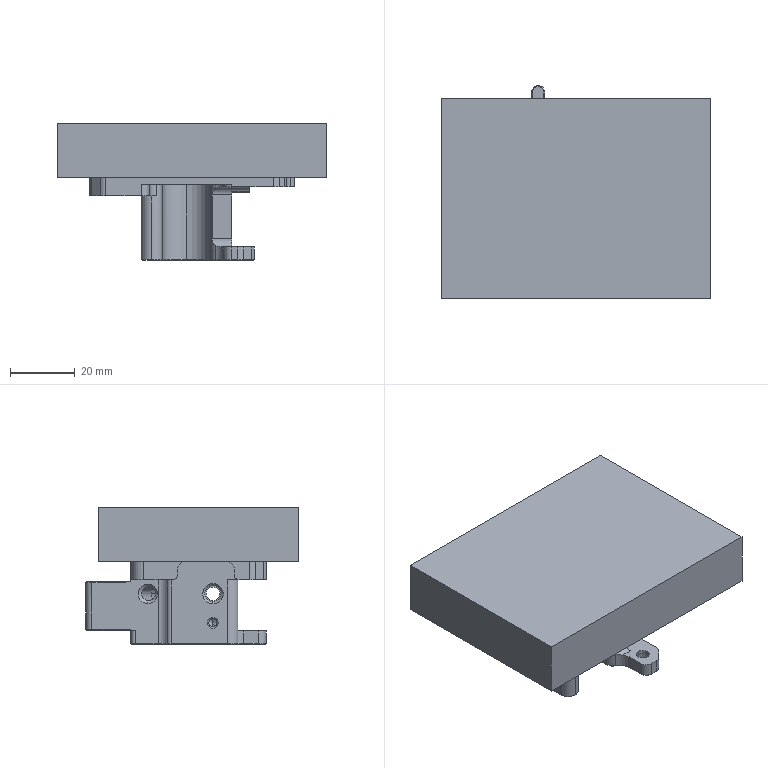NC program | NX | posted with a generic post | part box 83.5 x 66 x 42.45 mm
Whole program:
N10 G17 G21 G94 G90
(ADAPTIVE_MILLING_COPY , TOOL : D10)
N12 T10 M6
N14 G54
N16 G17 G0 G90 X-7.633 Y-11.797 B0. C0. S9500 M3
N18 G43 Z30. H10
N20 Z-19.85
N22 G94 G1 Z-20.85 F1000.
N24 X-5.94 Y-11.706 F3000.
N26 G3 X-4.993 Y-10.829 R1.017
N28 X-4.333 Y-6.187 R16.769
N30 X-4.228 Y3.51 R335.234
N32 G1 X-4.251 Y3.607
N34 X-4.284 Y3.702
N36 X-4.324 Y3.793
N38 X-4.371 Y3.884
N40 X-4.418 Y3.945
N42 X-4.486 Y4.064
N44 X-4.948 Y5.179
N46 X-4.974 Y5.275
N48 G3 X-6.744 Y5.833 R1.102
N50 X-7.136 Y4.797 Z-20.792 R1.208
N52 G1 X-7.132 Y3.95 Z-20.75
N54 X-7.069 Y-9.218
N56 Y-9.799 Z-20.779
N58 X-7.051 Y-10.38 Z-20.808
N60 G3 X-6.632 Y-11.082 Z-20.85 R1.13
N62 X-4.948 Y-10.629 R1.103
N64 X-3.658 Y-5.417 R13.194
N66 X-3.497 Y2.377 R65.836
N68 X-3.689 Y2.995 R2.088
N70 G1 X-4.418 Y3.945
N72 G3 X-5.825 Y4.237 R1.106
N74 X-6.392 Y3.195 Z-20.788 R1.124
N76 G1 X-6.401 Y2.446 Z-20.75
N78 X-6.528 Y-8.058
N80 X-6.529 Y-9.108 Z-20.803
N82 G3 X-6.038 Y-9.886 Z-20.85 R1.117
N84 X-4.486 Y-9.514 R1.104
N86 X-3.183 Y-6.164 R7.051
N88 X-2.791 Y1.51 R34.579
N90 X-3.587 Y2.892 R1.626
N92 G1 X-3.683 Y2.988
N94 X-3.744 Y3.067
N96 G3 X-5.105 Y3.383 R1.106
N98 X-5.72 Y2.355 Z-20.787 R1.123
N100 G1 X-5.753 Y1.621 Z-20.75
N102 X-6.168 Y-7.57
N104 X-6.203 Y-8.599 Z-20.802
N106 G3 X-5.719 Y-9.403 Z-20.85 R1.117
N108 X-4.236 Y-9.157 R1.104
N110 X-2.514 Y-5.381 R7.395
N112 X-2.122 Y0.886 R22.208
N114 X-2.63 Y2.157 R2.042
N116 G1 X-3.264 Y2.644
N118 G3 X-4.502 Y2.713 R1.108
N120 X-5.043 Y1.647 Z-20.787 R1.192
N122 G1 X-5.084 Y0.903 Z-20.75
N124 X-5.511 Y-6.724
N126 X-5.557 Y-7.759 Z-20.802
N128 G3 X-5.087 Y-8.565 Z-20.85 R1.117
N130 X-3.683 Y-8.438 R1.106
N132 X-2.144 Y-5.877 R4.961
N134 X-1.514 Y0.545 R15.572
N136 X-2.116 Y1.884 R2.124
N138 G1 X-2.197 Y1.942
N140 X-2.286 Y1.995
N142 X-2.511 Y2.089
N144 X-2.63 Y2.157
N146 X-2.709 Y2.218
N148 G3 X-3.915 Y2.305 R1.111
N150 X-4.491 Y1.259 Z-20.787 R1.193
N152 G1 X-4.559 Y0.516 Z-20.75
N154 X-5.192 Y-6.428
N156 X-5.276 Y-7.467 Z-20.802
N158 G3 X-4.841 Y-8.285 Z-20.85 R1.117
N160 X-3.508 Y-8.281 R1.108
N162 X-1.571 Y-5.568 R4.957
N164 X-0.975 Y0.436 R11.788
N166 X-1.771 Y1.782 R1.899
N168 G1 X-2.326 Y2.012
N170 G3 X-3.372 Y1.9 R1.115
N172 X-3.861 Y0.924 Z-20.793 R1.217
N174 G1 X-3.955 Y0.064 Z-20.75
N176 X-4.619 Y-5.981
N178 X-4.721 Y-7.021 Z-20.802
N180 G3 X-4.303 Y-7.846 Z-20.85 R1.117
N182 X-2.952 Y-7.854 R1.107
N184 X-0.956 Y-5.176 R5.002
N186 X-0.457 Y0.324 R9.629
N188 X-1.341 Y1.612 R1.726
N190 G1 X-1.397 Y1.627
N192 X-1.858 Y1.818
N194 G3 X-2.954 Y1.671 R1.112
N196 X-3.394 Y0.747 Z-20.797 R1.225
N198 G1 X-3.507 Y-0.188 Z-20.75
N200 X-4.163 Y-5.623
N202 X-4.232 Y-6.163 Z-20.777
N204 X-4.278 Y-6.704 Z-20.804
N206 G3 X-3.885 Y-7.498 Z-20.85 R1.127
N208 X-2.63 Y-7.607 R1.108
N210 X-0.743 Y-5.71 R3.753
N212 X0.048 Y0.209 R8.513
N214 X-0.831 Y1.488 R1.908
N216 G1 X-0.923 Y1.526
N218 X-1.019 Y1.555
N220 X-1.033 Y1.561
N222 X-1.265 Y1.592
N224 X-1.361 Y1.617
N226 G3 X-2.733 Y0.726 R1.103
N228 G1 X-3.834 Y-6.275
N230 G3 X-2.327 Y-7.462 R1.102
N232 X-0.136 Y-5.389 R3.838
N234 X0.494 Y0.234 R7.508
N236 X-0.552 Y1.49 R1.776
N238 G1 X-0.622 Y1.507
N240 X-1.118 Y1.572
N242 G3 X-2.349 Y0.647 R1.104
N244 G1 X-3.373 Y-6.089
N246 G3 X-1.865 Y-7.271 R1.102
N248 X0.473 Y-5.068 R3.97
N250 X0.89 Y0.36 R6.795
N252 X-0.664 Y1.512 R1.595
N254 X-1.897 Y0.57 R1.104
N256 G1 X-2.771 Y-5.866
N258 G3 X-1.397 Y-7.077 R1.102
N260 X0.586 Y-5.61 R3.118
N262 X1.352 Y0.309 R6.494
N264 X0.163 Y1.425 R1.608
N266 G1 X0.034
N268 X-0.034 Y1.429
N270 X-0.232 Y1.456
N272 G3 X-1.462 Y0.542 R1.104
N274 G1 X-2.494 Y-5.773
N276 G3 X-1.265 Y-7.042 R1.103
N278 X0.96 Y-5.68 R2.972
N280 X1.752 Y0.389 R6.179
N282 X0.59 Y1.425 R1.634
N284 G1 X0.09
N286 G3 X-0.994 Y0.517 R1.106
N288 G1 X-2.095 Y-5.707
N290 G3 X-0.868 Y-6.989 R1.103
N292 X1.45 Y-5.598 R3.065
N294 X2.193 Y0.372 R6.012
N296 X1.024 Y1.425 R1.704
N298 G1 X0.524
N300 G3 X-0.56 Y0.508 R1.106
N302 G1 X-1.601 Y-5.65
N304 G3 X-0.372 Y-6.924 R1.103
N306 X1.964 Y-5.486 R3.11
N308 X2.568 Y0.482 R5.809
N310 X0.942 Y1.425 R1.531
N312 X-0.142 Y0.511 R1.106
N314 G1 X-1.19 Y-5.596
N316 G3 X-0.034 Y-6.879 R1.103
N318 X2.175 Y-5.759 R2.764
N320 X2.987 Y0.515 R5.725
N322 X1.354 Y1.425 R1.535
N324 X0.272 Y0.524 R1.106
N326 G1 X-0.848 Y-5.576
N328 G3 X0.234 Y-6.875 R1.103
N330 X2.656 Y-5.708 R2.843
N332 X3.393 Y0.566 R5.65
N334 X1.814 Y1.425 R1.496
N336 X0.734 Y0.534 R1.106
N338 G1 X-0.446 Y-5.566
N340 G3 X0.634 Y-6.875 R1.103
N342 X3.071 Y-5.734 R2.871
N344 X3.852 Y0.532 R5.644
N346 X2.218 Y1.425 R1.527
N348 X1.138 Y0.534 R1.106
N350 G1 X-0.046 Y-5.566
N352 G3 X1.034 Y-6.875 R1.103
N354 X3.552 Y-5.69 R2.935
N356 X4.261 Y0.581 R5.604
N358 X2.681 Y1.425 R1.491
N360 X1.6 Y0.528 R1.106
N362 G1 X0.453 Y-5.572
N364 G3 X1.534 Y-6.875 R1.103
N366 X4.034 Y-5.645 R2.96
N368 X4.674 Y0.631 R5.585
N370 X3.147 Y1.425 R1.463
N372 X2.068 Y0.54 R1.106
N374 G1 X0.855 Y-5.56
N376 G3 X1.934 Y-6.875 R1.103
N378 X4.514 Y-5.604 R2.999
N380 X5.136 Y0.592 R5.596
N382 X3.553 Y1.425 R1.496
N384 X2.475 Y0.541 R1.106
N386 G1 X1.256 Y-5.559
N388 G3 X2.334 Y-6.875 R1.103
N390 X4.93 Y-5.639 R2.977
N392 X5.549 Y0.638 R5.575
N394 X3.957 Y1.425 R1.508
N396 X2.876 Y0.524 R1.106
N398 G1 X1.753 Y-5.576
N400 G3 X2.834 Y-6.875 R1.103
N402 X5.346 Y-5.673 R2.943
N404 X6.015 Y0.601 R5.602
N406 X4.419 Y1.425 R1.498
N408 X3.339 Y0.535 R1.106
N410 G1 X2.155 Y-5.565
N412 G3 X3.234 Y-6.875 R1.103
N414 X5.826 Y-5.629 R2.985
N416 X6.85 Y-3.596 R4.874
N418 X6.793 Y-0.5 R26.04
N420 X5.694 Y1.325 R2.496
N422 X4.909 Y1.425 R2.042
N424 X3.981 Y-0.266 R1.102
N426 G1 X4.822 Y-1.587
N428 G3 X6.85 Y-0.996 R1.101
N430 X6.524 Y0.842 R3.19
N432 X5.228 Y1.425 R1.276
N434 X4.451 Y-0.453 R1.101
N436 G1 X4.772 Y-0.775
N438 X5.104 Y-1.086
N440 G3 X6.85 Y-0.196 R1.101
N442 X6.431 Y1.164 R1.559
N444 X5.612 Y1.425 R1.3
N446 X6.501 Y-0.628 R-1.214
N448 X6.837 Y0.386 R1.243
N450 X6.122 Y1.342 R1.078
N452 G1 X5.147 Y1.12
N454 G3 X4.332 Y0.344 R1.112
N456 G1 X2.707 Y-5.471
N458 G3 X3.027 Y-6.582 R1.112
N460 X4.234 Y-6.872 R1.514
N462 X6.818 Y-4.735 R3.505
N464 X6.85 Y-3.537 R33.415
N466 X4.858 Y-2.893 R1.101
N468 G1 X3.243 Y-5.131
N470 G3 X4.134 Y-6.875 R1.101
N472 X6.782 Y-5.418 R2.78
N474 X6.85 Y-4.522 R3.2
N476 X4.928 Y-3.791 R1.101
N478 G1 X3.813 Y-5.044
N480 G3 X4.634 Y-6.875 R1.101
N482 X6.765 Y-5.853 R2.132
N484 X6.85 Y-5.106 R2.259
N486 X4.999 Y-4.302 R1.101
N488 G1 X4.575 Y-4.694
N490 X4.165 Y-5.101
N492 G3 X5.034 Y-6.875 R1.101
N494 X6.657 Y-6.303 R1.786
N496 X6.85 Y-5.437 R1.428
N498 X4.946 Y-4.686 R1.101
N500 G1 X4.518 Y-5.167
N502 G3 X5.434 Y-6.875 R1.102
N504 X6.84 Y-5.811 R1.191
N506 X6.075 Y-4.697 R1.015
N508 G1 X4.35 Y-4.281
N510 Z-17.85
N512 G0 Z30.
N514 X42.62 Y-2.812
N516 Z-19.85
N518 G1 Z-20.85 F1000.
N520 X40.185 Y-0.632 F3000.
N522 G3 X39.512 Y-0.375 R1.041
N524 X38.91 Y-3.194 R7.946
N526 X38.762 Y-8.987 R44.241
N528 G1 X39.491 Y-10.597
N530 G3 X41.373 Y-10.838 R1.102
N532 X41.574 Y-9.849 Z-20.798 R1.233
N534 G1 X41.465 Y-8.897 Z-20.75
N536 X40.781 Y-2.893
N538 X40.578 Y-1.204 Z-20.835
N540 X40.466 Y-0.928 Z-20.85
N542 G3 X39.512 Y-0.375 R1.112
N544 X38.58 Y-2.336 R4.017
N546 X38.108 Y-8.095 R19.474
N548 G1 X38.13 Y-8.192
N550 X38.161 Y-8.287
N552 X38.2 Y-8.379
N554 X38.246 Y-8.468
N556 X38.278 Y-8.519
N558 X38.896 Y-9.306
N560 G3 X40.86 Y-8.588 R1.101
N562 G1 X40.611 Y-1.437
N564 G3 X39.512 Y-0.375 R1.104
N566 X38.323 Y-1.93 R2.839
N568 X37.518 Y-7.422 R12.095
N570 X38.196 Y-8.415 R1.52
N572 G1 X38.32 Y-8.572
N574 G3 X40.284 Y-7.949 R1.101
N576 G1 X40.61 Y-1.531
N578 G3 X39.512 Y-0.375 R1.104
N580 X38.179 Y-1.509 R2.219
N582 X36.994 Y-6.984 R8.908
N584 X37.391 Y-7.788 R1.417
N586 G1 X37.951 Y-8.209
N588 G3 X39.698 Y-7.496 R1.102
N590 G1 X40.599 Y-1.642
N592 G3 X39.512 Y-0.375 R1.103
N594 X38.012 Y-1.255 R1.989
N596 X36.517 Y-6.7 R7.259
N598 X37.122 Y-7.586 R1.207
N600 G1 X37.442 Y-7.826
N602 G3 X39.172 Y-7.203 R1.102
N604 G1 X40.482 Y-1.731
N606 G3 X39.412 Y-0.375 R1.103
N608 X37.604 Y-1.284 R2.249
N610 X36.054 Y-6.387 R6.419
N612 X37.09 Y-7.568 R1.437
N614 X38.687 Y-6.915 R1.103
N616 G1 X40.169 Y-1.78
N618 G3 X39.112 Y-0.375 R1.103
N620 X37.121 Y-1.358 R2.527
N622 X35.641 Y-6.259 R5.807
N624 X36.777 Y-7.428 R1.47
N626 X38.232 Y-6.752 R1.104
N628 G1 X39.857 Y-1.819
N630 G3 X38.812 Y-0.375 R1.102
N632 X36.633 Y-1.413 R2.73
N634 X35.231 Y-6.123 R5.416
N636 X36.362 Y-7.262 R1.472
N638 X37.805 Y-6.618 R1.104
N640 G1 X39.545 Y-1.852
N642 G3 X38.512 Y-0.375 R1.102
N644 X36.08 Y-1.531 R2.915
N646 X34.855 Y-6.081 R5.051
N648 X35.962 Y-7.101 R1.343
N650 X37.401 Y-6.469 R1.104
N652 G1 X39.141 Y-1.864
N654 G3 X38.112 Y-0.375 R1.102
N656 X35.594 Y-1.569 R2.979
N658 X34.485 Y-6.038 R4.81
N660 X35.721 Y-7.028 R1.3
N662 X36.867 Y-6.359 R1.108
N664 G1 X38.727 Y-1.898
N666 G3 X37.712 Y-0.375 R1.102
N668 X35.111 Y-1.606 R3.015
N670 X34.083 Y-5.902 R4.665
N672 X35.466 Y-6.997 R1.392
N674 X36.631 Y-6.282 R1.106
N676 G1 X38.245 Y-1.852
N678 G3 X37.212 Y-0.375 R1.102
N680 X34.697 Y-1.573 R2.958
N682 X33.788 Y-6.055 R4.474
N684 X35.097 Y-6.953 R1.328
N686 X36.262 Y-6.235 R1.106
N688 G1 X37.846 Y-1.849
N690 G3 X36.812 Y-0.375 R1.102
N692 X34.221 Y-1.618 R2.966
N694 X33.415 Y-6.026 R4.406
N696 X34.776 Y-6.915 R1.379
N698 X35.954 Y-6.161 R1.106
N700 G1 X37.358 Y-1.813
N702 G3 X36.312 Y-0.375 R1.102
N704 X33.811 Y-1.592 R2.908
N706 X33.043 Y-6.002 R4.352
N708 X34.478 Y-6.879 R1.339
N710 X35.592 Y-6.114 R1.107
N712 G1 X36.96 Y-1.808
N714 G3 X35.912 Y-0.375 R1.103
N716 X33.282 Y-1.728 R2.926
N718 X32.766 Y-6.161 R4.226
N720 X34.115 Y-6.875 R1.284
N722 X35.168 Y-6.093 R1.108
N724 G1 X36.465 Y-1.793
N726 G3 X35.412 Y-0.375 R1.103
N728 X32.938 Y-1.633 R2.829
N730 X32.399 Y-6.148 R4.222
N732 X33.748 Y-6.875 R1.29
N734 X34.804 Y-6.085 R1.108
N736 G1 X36.067 Y-1.785
N738 G3 X35.012 Y-0.375 R1.103
N740 X32.537 Y-1.624 R2.8
N742 X32.076 Y-6.225 R4.166
N744 X33.031 Y-6.875 R1.276
N746 X34.064 Y-6.154 R1.108
N748 G1 X35.644 Y-1.855
N750 G3 X34.612 Y-0.375 R1.102
N752 X32.138 Y-1.619 R2.763
N754 X31.706 Y-6.225 R4.175
N756 X32.66 Y-6.875 R1.273
N758 G1 X33.36
N760 G3 X34.444 Y-5.964 R1.106
N762 G1 X35.195 Y-1.664
N764 G3 X34.112 Y-0.375 R1.103
N766 X31.801 Y-1.537 R2.68
N768 X31.335 Y-6.227 R4.202
N770 X32.291 Y-6.875 R1.282
N772 X33.336 Y-6.12 R1.108
N774 G1 X34.756 Y-1.82
N776 G3 X33.712 Y-0.375 R1.102
N778 X31.34 Y-1.615 R2.704
N780 X31.015 Y-6.31 R4.153
N782 X31.916 Y-6.875 R1.238
N784 X32.962 Y-6.115 R1.108
N786 G1 X34.358 Y-1.815
N788 G3 X33.312 Y-0.375 R1.102
N790 X30.941 Y-1.616 R2.695
N792 X30.15 Y-3.468 R4.553
N794 X30.361 Y-5.743 R6.35
N796 X31.475 Y-6.875 R1.607
N798 G1 X32.675
N800 G3 X33.774 Y-5.835 R1.104
N802 G1 X34.01 Y-1.535
N804 G3 X32.912 Y-0.375 R1.104
N806 X30.685 Y-1.44 R2.524
N808 X30.15 Y-2.478 R2.062
N810 G1 Y-3.478
N812 G3 X32.172 Y-4.077 R1.101
N814 G1 X33.484 Y-2.058
N816 G3 X32.633 Y-0.361 R1.102
N818 X30.191 Y-1.722 R2.337
N820 X30.15 Y-2.535 R7.597
N822 X32.097 Y-3.237 R1.101
N824 G1 X32.613 Y-2.623
N826 X33.109 Y-1.993
N828 G3 X32.234 Y-0.335 R1.102
N830 X30.201 Y-1.334 R1.806
N832 X30.15 Y-1.996 R2.134
N834 X32.084 Y-2.713 R1.101
N836 G1 X32.407 Y-2.34
N838 X32.716 Y-1.956
N840 G3 X31.99 Y-0.302 R1.102
N842 X30.159 Y-1.2 R1.423
N844 G1 X30.15 Y-1.315
N846 Y-1.515
N848 G3 X31.695 Y-0.244 R-1.295
N850 X30.155 Y-1.255 R1.153
N852 X32.247 Y-1.34 R-1.047
N854 X30.921 Y-0.241 R1.094
N856 X30.162 Y-1.155 R1.124
N858 G1 X30.15 Y-1.315
N860 Y-4.568
N862 G3 X30.365 Y-6.233 R3.413
N864 X31.488 Y-6.875 R1.101
N866 X32.357 Y-5.101 R1.101
N868 G1 X31.996 Y-4.66
N870 G3 X30.15 Y-5.468 R1.101
N872 X31.115 Y-6.852 R1.188
N874 X32.223 Y-6.109 R1.015
N876 G1 X32.682 Y-4.375
N878 Z-17.85
N880 G0 Z30.
N882 X33.104 Y-2.875
N884 Z-18.35
N886 G1 Z-19.35 F1000.
N888 X31.654 Y-0.499 F3000.
N890 G3 X31.163 Y-0.086 R1.052
N892 X29.911 Y-0.971 R1.106
N894 X29.52 Y-5.518 R10.628
N896 X30.478 Y-6.827 R1.624
N898 G1 X30.575 Y-6.852
N900 X30.673 Y-6.87
N902 X30.693 Y-6.875
N904 X30.893
N906 G3 X31.992 Y-5.743 R1.104
N908 G1 X31.858 Y-1.078
N910 G3 X31.163 Y-0.086 R1.108
N912 X29.892 Y-0.598 R1.041
N914 X29.125 Y-5.603 R6.555
N916 X30.18 Y-6.843 R1.696
N918 G1 X30.278 Y-6.864
N920 X30.314 Y-6.875
N922 X30.714
N924 G3 X31.814 Y-5.764 R1.104
N926 G1 X31.766 Y-1.061
N928 G3 X31.071 Y-0.049 R1.108
N930 X29.743 Y-0.481 R1.168
N932 X28.815 Y-5.841 R5.414
N934 X30.361 Y-6.875 R1.469
N936 X31.46 Y-5.824 R1.104
N938 G1 X31.672 Y-1.085
N940 G3 X30.978 Y-0.013 R1.108
N942 X29.524 Y-0.411 R1.358
N944 X28.519 Y-6.041 R4.94
N946 X29.984 Y-6.875 R1.396
N948 X31.078 Y-5.889 R1.106
N950 G1 X31.574 Y-1.112
N952 G3 X30.885 Y0.024 R1.108
N954 X29.309 Y-0.301 R1.492
N956 X28.164 Y-6.116 R4.763
N958 X29.6 Y-6.875 R1.368
N960 X30.689 Y-5.931 R1.106
N962 G1 X31.383 Y-1.081
N964 G3 X30.699 Y0.098 R1.106
N966 X29.016 Y-0.225 R1.662
N968 X27.795 Y-6.171 R4.709
N970 X29.208 Y-6.875 R1.357
N972 X30.29 Y-5.973 R1.106
N974 G1 X31.19 Y-1.049
N976 G3 X30.513 Y0.171 R1.106
N978 X28.724 Y-0.13 R1.813
N980 X27.42 Y-6.21 R4.682
N982 X28.899 Y-6.875 R1.443
N984 X29.977 Y-5.996 R1.106
N986 G1 X31. Y-0.998
N988 G3 X30.327 Y0.245 R1.106
N990 X28.392 Y-0.042 R1.938
N992 X26.95 Y-6.104 R4.744
N994 X28.4 Y-6.875 R1.384
N996 X29.468 Y-6.039 R1.107
N998 G1 X30.732 Y-0.932
N1000 G3 X30.187 Y0.3 R1.107
N1002 X28.353 Y0.234 R1.818
N1004 X26.554 Y-6.12 R4.77
N1006 X28.094 Y-6.875 R1.458
N1008 X29.159 Y-6.05 R1.107
N1010 G1 X30.509 Y-0.814
N1012 G3 X30.078 Y0.359 R1.108
N1014 X28.272 Y0.469 R1.761
N1016 X25.602 Y-3.585 R4.701
N1018 X26.497 Y-6.561 R3.849
N1020 X27.595 Y-6.875 R1.385
N1022 X28.645 Y-6.105 R1.108
N1024 G1 X30.329 Y-0.754
N1026 G3 X29.915 Y0.475 R1.108
N1028 X27.921 Y0.602 R1.932
N1030 X25.17 Y-3.93 R4.894
N1032 X26.198 Y-6.655 R3.571
N1034 X27.277 Y-6.875 R1.642
N1036 X28.319 Y-6.126 R1.108
N1038 G1 X30.159 Y-0.66
N1040 G3 X29.751 Y0.59 R1.108
N1042 X27.668 Y0.786 R2.019
N1044 X24.751 Y-3.756 R5.003
N1046 X25.728 Y-6.607 R3.797
N1048 X26.865 Y-6.875 R1.56
N1050 X27.901 Y-6.144 R1.108
N1052 G1 X29.908 Y-0.504
N1054 G3 X29.506 Y0.763 R1.108
N1056 X27.42 Y0.978 R2.06
N1058 X24.358 Y-3.266 R5.054
N1060 X25.248 Y-6.542 R4.104
N1062 X26.457 Y-6.875 R1.491
N1064 X27.488 Y-6.16 R1.108
N1066 G1 X29.657 Y-0.347
N1068 G3 X29.261 Y0.936 R1.107
N1070 X27.078 Y1.147 R2.161
N1072 X23.903 Y-3.562 R5.236
N1074 X24.9 Y-6.607 R3.925
N1076 X26.037 Y-6.875 R1.56
N1078 X27.061 Y-6.176 R1.108
N1080 G1 X29.406 Y-0.191
N1082 G3 X29.016 Y1.109 R1.107
N1084 X28.201 Y1.425 R1.402
N1086 X24.604 Y-0.338 R3.962
N1088 X24.004 Y-6.003 R5.379
N1090 X25.634 Y-6.875 R1.506
N1092 X26.686 Y-6.097 R1.108
N1094 G1 X28.553 Y0.003
N1096 G3 X27.501 Y1.425 R1.103
N1098 X24.366 Y-0.02 R3.589
N1100 X23.539 Y-5.925 R5.498
N1102 X25.205 Y-6.875 R1.528
N1104 X26.264 Y-6.07 R1.108
N1106 G1 X27.961 Y0.03
N1108 G3 X26.901 Y1.425 R1.103
N1110 X23.945 Y0.051 R3.398
N1112 X23.122 Y-5.945 R5.532
N1114 X24.777 Y-6.875 R1.529
N1116 X25.844 Y-6.042 R1.107
N1118 G1 X27.368 Y0.058
N1120 G3 X26.301 Y1.425 R1.103
N1122 X23.523 Y0.111 R3.261
N1124 X22.659 Y-5.886 R5.604
N1126 X24.343 Y-6.875 R1.563
N1128 X25.413 Y-6.031 R1.106
N1130 G1 X26.871 Y0.069
N1132 G3 X25.801 Y1.425 R1.103
N1134 X23.103 Y0.164 R3.171
N1136 X22.245 Y-5.919 R5.603
N1138 X23.924 Y-6.875 R1.549
N1140 X24.998 Y-6.017 R1.106
N1142 G1 X26.374 Y0.083
N1144 G3 X25.301 Y1.425 R1.103
N1146 X22.684 Y0.213 R3.093
N1148 X21.831 Y-5.954 R5.594
N1150 X23.482 Y-6.875 R1.532
N1152 X24.557 Y-6.007 R1.106
N1154 G1 X25.876 Y0.093
N1156 G3 X24.801 Y1.425 R1.103
N1158 X22.2 Y0.184 R3.074
N1160 X21.419 Y-5.99 R5.576
N1162 X23.053 Y-6.875 R1.516
N1164 X24.131 Y-5.995 R1.106
N1166 G1 X25.379 Y0.105
N1168 G3 X24.301 Y1.425 R1.103
N1170 X21.78 Y0.227 R3.03
N1172 X21.006 Y-6.032 R5.578
N1174 X22.614 Y-6.875 R1.5
N1176 X23.69 Y-6.002 R1.106
N1178 G1 X24.977 Y0.098
N1180 G3 X23.901 Y1.425 R1.103
N1182 X21.297 Y0.194 R3.043
N1184 X20.542 Y-5.987 R5.605
N1186 X22.176 Y-6.875 R1.521
N1188 X23.255 Y-5.992 R1.106
N1190 G1 X24.48 Y0.108
N1192 G3 X23.401 Y1.425 R1.103
N1194 X20.88 Y0.233 R3.004
N1196 X20.13 Y-6.031 R5.59
N1198 X21.742 Y-6.875 R1.506
N1200 X22.819 Y-5.997 R1.106
N1202 G1 X24.078 Y0.103
N1204 G3 X23.001 Y1.425 R1.103
N1206 X20.398 Y0.196 R3.025
N1208 X19.667 Y-5.989 R5.617
N1210 X21.302 Y-6.875 R1.525
N1212 X22.382 Y-5.987 R1.106
N1214 G1 X23.58 Y0.113
N1216 G3 X22.501 Y1.425 R1.103
N1218 X19.916 Y0.157 R3.031
N1220 X19.255 Y-6.034 R5.588
N1222 X20.866 Y-6.875 R1.508
N1224 X21.944 Y-5.993 R1.106
N1226 G1 X23.179 Y0.107
N1228 G3 X22.101 Y1.425 R1.103
N1230 X19.5 Y0.192 R3.018
N1232 X18.845 Y-6.08 R5.573
N1234 X20.432 Y-6.875 R1.502
N1236 X21.512 Y-5.982 R1.106
N1238 G1 X22.681 Y0.118
N1240 G3 X21.601 Y1.425 R1.103
N1242 X19.084 Y0.227 R2.983
N1244 X18.381 Y-6.042 R5.591
N1246 X19.987 Y-6.875 R1.508
N1248 X21.066 Y-5.99 R1.106
N1250 G1 X22.28 Y0.11
N1252 G3 X21.201 Y1.425 R1.103
N1254 X18.603 Y0.189 R3.011
N1256 X17.917 Y-6.001 R5.618
N1258 X19.559 Y-6.875 R1.524
N1260 X20.64 Y-5.977 R1.106
N1262 G1 X21.782 Y0.123
N1264 G3 X20.701 Y1.425 R1.103
N1266 X18.187 Y0.224 R2.972
N1268 X17.505 Y-6.049 R5.598
N1270 X19.106 Y-6.875 R1.505
N1272 X20.185 Y-5.986 R1.106
N1274 G1 X21.381 Y0.114
N1276 G3 X20.301 Y1.425 R1.103
N1278 X17.707 Y0.183 R3.001
N1280 X17.041 Y-6.009 R5.603
N1282 X18.677 Y-6.875 R1.521
N1284 X19.759 Y-5.974 R1.106
N1286 G1 X20.883 Y0.126
N1288 G3 X19.801 Y1.425 R1.103
N1290 X17.292 Y0.216 R2.959
N1292 X16.028 Y-2.678 R5.781
N1294 X18.007 Y-3.488 R1.101
N1296 G1 X20.293 Y-0.318
N1298 G3 X19.401 Y1.425 R1.101
N1300 X16.812 Y0.175 R2.981
N1302 X16.031 Y-1.1 R6.798
N1304 X17.815 Y-2.324 R1.1
N1306 G1 X19.68 Y-0.451
N1308 G3 X18.901 Y1.425 R1.101
N1310 X16.396 Y0.208 R2.953
N1312 G1 X16.332 Y0.131
N1314 X16.271 Y0.052
N1316 X16.212 Y-0.028
N1318 X16.155 Y-0.111
N1320 X16.101 Y-0.195
N1322 X16.05 Y-0.281
N1324 X16.005 Y-0.371
N1326 X15.951 Y-0.454
N1328 X15.887 Y-0.531
N1330 X15.815 Y-0.601
N1332 G2 X13.693 Y-1.037 R3.605
N1334 X9.481 Y0.413 R9.233
N1336 G3 X7.632 Y1.399 R13.696
N1338 G1 X7.534 Y1.418
N1340 X7.47 Y1.425
N1342 X6.07
N1344 G3 X5.314 Y-0.255 R1.011
N1346 G1 X5.584 Y-0.561
N1348 X5.866 Y-0.857
N1350 G3 X6.498 Y-1.079 R1.05
N1352 G1 Z-16.35
N1354 G0 Z30.
N1356 X18.779 Y-1.087
N1358 Z-18.35
N1360 G1 Z-19.35 F1000.
N1362 G3 X19.659 Y0.42 R1.012 F3000.
N1364 G1 X19.296 Y1.039
N1366 G3 X18.501 Y1.425 R1.026
N1368 X16.855 Y1.087 R3.428
N1370 G2 X11.338 Y1.163 R9.468
N1372 G1 X11.049 Y1.243
N1374 X10.568 Y1.381
N1376 X10.471 Y1.405
N1378 X10.373 Y1.422
N1380 X10.342 Y1.425
N1382 X7.442
N1384 G3 X6.344 Y0.323 R1.1
N1386 X7.442 Y-0.775 R1.1
N1388 G1 X18.001
N1390 G3 X19.099 Y0.327 R1.1
N1392 X18.001 Y1.425 R1.1
N1394 G1 X10.301
N1396 G3 X9.393 Y0.946 R1.116
N1398 G1 X5.223 Y-5.154
N1400 G3 X6.131 Y-6.875 R1.101
N1402 X6.991 Y-6.128 R1.118
N1404 G2 X8.68 Y-4.837 R2.414
N1406 X13.443 Y-5.402 R6.92
N1408 G1 X13.534 Y-5.443
N1410 X13.715 Y-5.527
N1412 X13.985 Y-5.658
N1414 X14.253 Y-5.793
N1416 X14.519 Y-5.932
N1418 X14.872 Y-6.12
N1420 X15.136 Y-6.262
N1422 X15.401 Y-6.403
N1424 X15.579 Y-6.495
N1426 X15.757 Y-6.586
N1428 X15.846 Y-6.631
N1430 X16.027 Y-6.718
N1432 X16.117 Y-6.759
N1434 X16.209 Y-6.8
N1436 X16.304 Y-6.832
N1438 G3 X18.227 Y-6.875 R12.574
N1440 X19.325 Y-5.773 R1.1
N1442 X18.227 Y-4.675 R1.1
N1444 G1 X6.131
N1446 G3 X5.033 Y-5.777 R1.1
N1448 X6.131 Y-6.875 R1.1
N1450 X7.182 Y-6.581 R3.325
N1452 G2 X12.804 Y-6.695 R10.069
N1454 G1 X13.094 Y-6.772
N1456 X13.383 Y-6.851
N1458 X13.481 Y-6.869
N1460 X13.538 Y-6.875
N1462 X16.538
N1464 G3 X17.636 Y-5.773 R1.1
N1466 X16.538 Y-4.675 R1.1
N1468 G1 X6.231
N1470 G3 X5.133 Y-5.777 R1.1
N1472 X6.231 Y-6.875 R1.1
N1474 G1 X13.631
N1476 G3 X14.63 Y-5.716 R1.014
N1478 G1 X14.447 Y-4.485
N1480 Z-16.35
N1482 G0 Z30.
N1484 X39.329 Y-1.071
N1486 Z-12.482
N1488 G1 Z-13.482 F1000.
N1490 X39.004 Y0.607 F3000.
N1492 G3 X38.012 Y1.425 R1.017
N1494 G2 X31.62 Y1.402 R10.217
N1496 G1 X31.521 Y1.42
N1498 X31.473 Y1.425
N1500 X28.473
N1502 G3 X27.375 Y0.323 R1.1
N1504 X28.473 Y-0.775 R1.1
N1506 G1 X38.012
N1508 G3 X39.11 Y0.327 R1.1
N1510 X38.012 Y1.425 R1.1
N1512 G1 X31.412
N1514 G3 X30.408 Y0.521 R1.015
N1516 G1 X30.24 Y-1.072
N1518 Z-10.482
N1520 G0 Z30.
N1522 M5
(DRILLING_COPY_1_COPY_COPY , TOOL : D4A45)
N1524 T07 M6
N1526 G54
N1528 G17 G0 G90 X16.52 Y-0.525 B0. C0. S5000 M3
N1530 G43 Z30. H7
N1532 G94 G81 G98 Z-21.15 F250. R-16.5
N1534 G80
N1536 G0 X16.52 Y-0.525 Z30.
N1538 M5
(DRILLING_COPY_COPY_1_1_COPY_COPY , TOOL : 4.2ZT)
N1540 T14 M6
N1542 G54
N1544 G17 G0 G90 X16.52 Y-0.525 B0. C0. S2000 M3
N1546 G43 Z30. H14
N1548 G94 G83 G98 Z-28.762 F120. Q2. R-16.5
N1550 G80
N1552 G0 X16.52 Y-0.525 Z30.
N1554 M5
(ZLEVEL_PROFILE_COPY_1_COPY_1_COPY_1_1_COPY_COPY_COPY_1_COPY_1 , TOOL : D4)
N1556 T04 M6
N1558 G54
N1560 G17 G0 G90 X31.192 Y2.422 B0. C0. S9500 M3
N1562 G43 Z30. H4
N1564 Z-14.4
N1566 G94 G1 X31.316 Y3.026 F800.
N1568 G3 X31.189 Y3.406 R0.4
N1570 G2 X30.558 Y4.275 R2.5 F1400.
N1572 G3 X30.1 Y4.575 R0.5
N1574 G1 X28.627
N1576 G3 X28.281 Y4.375 R0.4
N1578 G1 X27.934 Y3.775
N1580 G0 X31.192 Y2.422 Z-14.8
N1582 G1 X31.316 Y3.026 F800.
N1584 G3 X31.189 Y3.406 R0.4
N1586 G2 X30.558 Y4.275 R2.5 F1400.
N1588 G3 X30.1 Y4.575 R0.5
N1590 G1 X28.627
N1592 G3 X28.281 Y4.375 R0.4
N1594 G1 X27.934 Y3.775
N1596 G0 X31.192 Y2.422 Z-15.2
N1598 G1 X31.316 Y3.026 F800.
N1600 G3 X31.189 Y3.406 R0.4
N1602 G2 X30.558 Y4.275 R2.5 F1400.
N1604 G3 X30.1 Y4.575 R0.5
N1606 G1 X28.627
N1608 G3 X28.281 Y4.375 R0.4
N1610 G1 X27.934 Y3.775
N1612 G0 X31.192 Y2.422 Z-15.6
N1614 G1 X31.316 Y3.026 F800.
N1616 G3 X31.189 Y3.406 R0.4
N1618 G2 X30.558 Y4.275 R2.5 F1400.
N1620 G3 X30.1 Y4.575 R0.5
N1622 G1 X28.627
N1624 G3 X28.281 Y4.375 R0.4
N1626 G1 X27.934 Y3.775
N1628 G0 X31.192 Y2.422 Z-16.
N1630 G1 X31.316 Y3.026 F800.
N1632 G3 X31.189 Y3.406 R0.4
N1634 G2 X30.558 Y4.275 R2.5 F1400.
N1636 G3 X30.1 Y4.575 R0.5
N1638 G1 X28.627
N1640 G3 X28.281 Y4.375 R0.4
N1642 G1 X27.934 Y3.775
N1644 G0 X31.192 Y2.422 Z-16.4
N1646 G1 X31.316 Y3.026 F800.
N1648 G3 X31.189 Y3.406 R0.4
N1650 G2 X30.558 Y4.275 R2.5 F1400.
N1652 G3 X30.1 Y4.575 R0.5
N1654 G1 X28.627
N1656 G3 X28.281 Y4.375 R0.4
N1658 G1 X27.934 Y3.775
N1660 G0 X31.192 Y2.422 Z-16.8
N1662 G1 X31.316 Y3.026 F800.
N1664 G3 X31.189 Y3.406 R0.4
N1666 G2 X30.558 Y4.275 R2.5 F1400.
N1668 G3 X30.1 Y4.575 R0.5
N1670 G1 X28.627
N1672 G3 X28.281 Y4.375 R0.4
N1674 G1 X27.934 Y3.775
N1676 G0 X31.192 Y2.422 Z-17.199
N1678 G1 X31.316 Y3.026 F800.
N1680 G3 X31.189 Y3.406 R0.4
N1682 G2 X30.558 Y4.275 R2.5 F1400.
N1684 G3 X30.1 Y4.575 R0.5
N1686 G1 X28.627
N1688 G3 X28.281 Y4.375 R0.4
N1690 G1 X27.934 Y3.775
N1692 G0 X31.192 Y2.422 Z-17.599
N1694 G1 X31.316 Y3.026 F800.
N1696 G3 X31.189 Y3.406 R0.4
N1698 G2 X30.558 Y4.275 R2.5 F1400.
N1700 G3 X30.1 Y4.575 R0.5
N1702 G1 X28.627
N1704 G3 X28.281 Y4.375 R0.4
N1706 G1 X27.934 Y3.775
N1708 G0 X31.192 Y2.422 Z-17.999
N1710 G1 X31.316 Y3.026 F800.
N1712 G3 X31.189 Y3.406 R0.4
N1714 G2 X30.558 Y4.275 R2.5 F1400.
N1716 G3 X30.1 Y4.575 R0.5
N1718 G1 X28.627
N1720 G3 X28.281 Y4.375 R0.4
N1722 G1 X27.934 Y3.775
N1724 G0 X31.192 Y2.422 Z-18.375
N1726 G1 X31.316 Y3.026 F800.
N1728 G3 X31.189 Y3.406 R0.4
N1730 G2 X30.558 Y4.275 R2.5 F1400.
N1732 G3 X30.1 Y4.575 R0.5
N1734 G1 X28.627
N1736 G3 X28.281 Y4.375 R0.4
N1738 G1 X27.934 Y3.775
N1740 G0 X31.192 Y2.422 Z-18.75
N1742 G1 X31.316 Y3.026 F800.
N1744 G3 X31.189 Y3.406 R0.4
N1746 G2 X30.558 Y4.275 R2.5 F1400.
N1748 G3 X30.1 Y4.575 R0.5
N1750 G1 X28.627
N1752 G3 X28.281 Y4.375 R0.4
N1754 G1 X27.934 Y3.775
N1756 G0 X31.192 Y2.422 Z-19.125
N1758 G1 X31.316 Y3.026 F800.
N1760 G3 X31.189 Y3.406 R0.4
N1762 G2 X30.558 Y4.275 R2.5 F1400.
N1764 G3 X30.1 Y4.575 R0.5
N1766 G1 X28.627
N1768 G3 X28.281 Y4.375 R0.4
N1770 G1 X27.934 Y3.775
N1772 G0 X31.192 Y2.422 Z-19.5
N1774 G1 X31.316 Y3.026 F800.
N1776 G3 X31.189 Y3.406 R0.4
N1778 G2 X30.558 Y4.275 R2.5 F1400.
N1780 G3 X30.1 Y4.575 R0.5
N1782 G1 X28.627
N1784 G3 X28.281 Y4.375 R0.4
N1786 G1 X27.934 Y3.775
N1788 G0 X32.071 Y2.068 Z-19.85
N1790 G1 X32.018 Y2.683 F800.
N1792 G3 X31.789 Y3.011 R0.4
N1794 G2 X30.558 Y4.275 R2.5 F1400.
N1796 G3 X30.1 Y4.575 R0.5
N1798 G1 X27.5
N1800 G3 X27. Y4.075 R0.5
N1802 G1 Y0.418
N1804 G3 X27.2 Y0.071 R0.4
N1806 G1 X27.8 Y-0.275
N1808 G0 X32.071 Y2.068 Z-20.177
N1810 G1 X32.018 Y2.683 F800.
N1812 G3 X31.789 Y3.011 R0.4
N1814 G2 X30.558 Y4.275 R2.5 F1400.
N1816 G3 X30.1 Y4.575 R0.5
N1818 G1 X27.5
N1820 G3 X27. Y4.075 R0.5
N1822 G1 Y0.418
N1824 G3 X27.2 Y0.071 R0.4
N1826 G1 X27.8 Y-0.275
N1828 G0 X32.071 Y2.068 Z-20.474
N1830 G1 X32.018 Y2.683 F800.
N1832 G3 X31.789 Y3.011 R0.4
N1834 G2 X30.558 Y4.275 R2.5 F1400.
N1836 G3 X30.1 Y4.575 R0.5
N1838 G1 X27.5
N1840 G3 X27. Y4.075 R0.5
N1842 G1 Y0.418
N1844 G3 X27.2 Y0.071 R0.4
N1846 G1 X27.8 Y-0.275
N1848 G0 X32.071 Y2.068 Z-20.74
N1850 G1 X32.018 Y2.683 F800.
N1852 G3 X31.789 Y3.011 R0.4
N1854 G2 X30.558 Y4.275 R2.5 F1400.
N1856 G3 X30.1 Y4.575 R0.5
N1858 G1 X27.5
N1860 G3 X27. Y4.075 R0.5
N1862 G1 Y0.418
N1864 G3 X27.2 Y0.071 R0.4
N1866 G1 X27.8 Y-0.275
N1868 G0 X32.071 Y2.068 Z-20.879
N1870 G1 X32.018 Y2.683 F800.
N1872 G3 X31.789 Y3.011 R0.4
N1874 G2 X30.558 Y4.275 R2.5 F1400.
N1876 G3 X30.1 Y4.575 R0.5
N1878 G1 X27.5
N1880 G3 X27. Y4.075 R0.5
N1882 G1 Y0.418
N1884 G3 X27.2 Y0.071 R0.4
N1886 G1 X27.8 Y-0.275
N1888 G0 X32.071 Y2.068 Z-21.
N1890 G1 X32.018 Y2.683 F800.
N1892 G3 X31.789 Y3.011 R0.4
N1894 G2 X30.558 Y4.275 R2.5 F1400.
N1896 G3 X30.1 Y4.575 R0.5
N1898 G1 X27.5
N1900 G3 X27. Y4.075 R0.5
N1902 G1 Y0.418
N1904 G3 X27.2 Y0.071 R0.4
N1906 G1 X27.8 Y-0.275
N1908 G0 Z30.
N1910 Y-6.179
N1912 Z-19.85
N1914 G1 X27.2 Y-6.526 F800.
N1916 G3 X27. Y-6.872 R0.4
N1918 G1 Y-9.525 F1400.
N1920 G3 X27.5 Y-10.025 R0.5
N1922 G1 X30.153
N1924 G3 X30.499 Y-9.825 R0.4
N1926 G1 X30.846 Y-9.225
N1928 G0 X27.8 Y-6.179 Z-20.177
N1930 G1 X27.2 Y-6.526 F800.
N1932 G3 X27. Y-6.872 R0.4
N1934 G1 Y-9.525 F1400.
N1936 G3 X27.5 Y-10.025 R0.5
N1938 G1 X30.153
N1940 G3 X30.499 Y-9.825 R0.4
N1942 G1 X30.846 Y-9.225
N1944 G0 X27.8 Y-6.179 Z-20.474
N1946 G1 X27.2 Y-6.526 F800.
N1948 G3 X27. Y-6.872 R0.4
N1950 G1 Y-9.525 F1400.
N1952 G3 X27.5 Y-10.025 R0.5
N1954 G1 X30.153
N1956 G3 X30.499 Y-9.825 R0.4
N1958 G1 X30.846 Y-9.225
N1960 G0 X27.8 Y-6.179 Z-20.74
N1962 G1 X27.2 Y-6.526 F800.
N1964 G3 X27. Y-6.872 R0.4
N1966 G1 Y-9.525 F1400.
N1968 G3 X27.5 Y-10.025 R0.5
N1970 G1 X30.153
N1972 G3 X30.499 Y-9.825 R0.4
N1974 G1 X30.846 Y-9.225
N1976 G0 X27.8 Y-6.179 Z-20.879
N1978 G1 X27.2 Y-6.526 F800.
N1980 G3 X27. Y-6.872 R0.4
N1982 G1 Y-9.525 F1400.
N1984 G3 X27.5 Y-10.025 R0.5
N1986 G1 X30.153
N1988 G3 X30.499 Y-9.825 R0.4
N1990 G1 X30.846 Y-9.225
N1992 G0 X27.8 Y-6.179 Z-21.
N1994 G1 X27.2 Y-6.526 F800.
N1996 G3 X27. Y-6.872 R0.4
N1998 G1 Y-9.525 F1400.
N2000 G3 X27.5 Y-10.025 R0.5
N2002 G1 X30.153
N2004 G3 X30.499 Y-9.825 R0.4
N2006 G1 X30.846 Y-9.225
N2008 G0 Z30.
(FLOOR_WALL_1_1_COPY_1_COPY , TOOL : D4)
N2010 X43.418 Y1.588
N2012 Z-12.5
N2014 G1 Z-14. F1000.
N2016 X42.846 Y2.578
N2018 G3 X42.5 Y2.778 R0.4
N2020 G1 X32.727
N2022 G2 X30.5 Y4.375 R2.548
N2024 G1 X42.5
N2026 G2 X42.846 Y4.175 R0.4
N2028 G1 X43.925 Y2.307
N2030 Z-12.5
N2032 G0 Z30.
N2034 X43.963 Y2.442
N2036 Z-12.5
N2038 G1 Z-14.
N2040 X42.846 Y4.375
N2042 G3 X42.5 Y4.575 R0.4
N2044 G1 X30.276
N2046 G3 X29.929 Y4.375 R0.4
N2048 G1 X29.179 Y3.075
N2050 Z-12.5
N2052 G0 Z30.
N2054 X38.197 Y1.275
N2056 Z-19.5
N2058 G1 Z-21.
N2060 X36.497 Y2.229
N2062 G3 X36.697 Y2.575 R0.4
N2064 G1 Y-9.825
N2066 X34.798
N2068 Y2.575
N2070 X32.898
N2072 Y-9.825
N2074 X30.999
N2076 Y3.309
N2078 G2 X30.375 Y4.195 R2.7
N2080 G3 X30.1 Y4.375 R0.3
N2082 G1 X29.099
N2084 Y-9.825
N2086 X27.5
N2088 G2 X27.2 Y-9.528 R0.3
N2090 G1 Y4.078
N2092 G2 X27.3 Y4.251 R0.2
N2094 G1 Z-19.5
N2096 G0 Z30.
N2098 X38.197 Y0.577
N2100 Z-19.5
N2102 G1 Z-21.
N2104 X37.044 Y2.575
N2106 G3 X36.697 Y2.775 R0.4
N2108 G1 X32.85
N2110 G2 X30.558 Y4.275 R2.5
N2112 G3 X30.1 Y4.575 R0.5
N2114 G1 X27.5
N2116 G3 X27. Y4.075 R0.5
N2118 G1 Y-9.525
N2120 G3 X27.5 Y-10.025 R0.5
N2122 G1 X36.697
N2124 G3 X37.044 Y-9.825 R0.4
N2126 G1 X38.197 Y-7.827
N2128 Z-19.5
N2130 G0 Z30.
N2132 X8.5 Y3.075
N2134 Z-18.
N2136 G1 Z-19.5
N2138 X10.249 Y4.172
N2140 G3 X9.902 Y4.372 R0.4
N2142 G1 X27.098
N2144 X27. Y2.597
N2146 X10.
N2148 Y0.823
N2150 X27.
N2152 Y-0.952
N2154 X10.
N2156 Y-2.726
N2158 X27.
N2160 Y-4.501
N2162 X10.
N2164 Y-6.276
N2166 X27.
N2168 Y-8.05
N2170 X10.
N2172 X9.9 Y-9.825
N2174 X27.1
N2176 G3 X27.446 Y-9.625 R0.4
N2178 G1 X28.5 Y-7.8
N2180 Z-18.
N2182 G0 Z30.
N2184 Y2.938
N2186 Z-18.
N2188 G1 Z-19.5
N2190 X27.671 Y4.375
N2192 G3 X27.324 Y4.575 R0.4
N2194 G1 X9.676
N2196 G3 X9.329 Y4.375 R0.4
N2198 G1 X8.5 Y2.938
N2200 Z-18.
N2202 G0 Z30.
N2204 Y-8.388
N2206 Z-18.
N2208 G1 Z-19.5
N2210 X9.329 Y-9.825
N2212 G3 X9.676 Y-10.025 R0.4
N2214 G1 X27.324
N2216 G3 X27.671 Y-9.825 R0.4
N2218 G1 X28.5 Y-8.388
N2220 Z-18.
N2222 G0 Z30.
N2224 M5
(TOOLCOMP15_1 , TOOL : D4.05XYD)
N2226 T15 M6
N2228 G54
N2230 G17 G0 G90 X16.52 Y-0.525 B0. C0. S3000 M3
N2232 G43 Z30. H15
N2234 Z-18.328
N2236 G42 G94 G1 X16.423 Y-0.5 F800. D15
N2238 G2 X16.52 Y-0.05 Z-18.5 R0.236
N2240 X16.52 Y-0.05 Z-19.3 I0. J-0.475
N2242 X16.52 Y-0.05 Z-20.1 I0. J-0.475
N2244 X16.52 Y-0.05 Z-20.9 I0. J-0.475
N2246 X16.52 Y-0.05 Z-21.7 I0. J-0.475
N2248 X16.52 Y-0.05 Z-22.5 I0. J-0.475
N2250 X16.52 Y-0.05 Z-23.3 I0. J-0.475
N2252 X16.52 Y-0.05 Z-24.1 I0. J-0.475
N2254 X16.52 Y-0.05 Z-24.9 I0. J-0.475
N2256 X16.52 Y-0.05 Z-25.7 I0. J-0.475
N2258 X16.856 Y-0.861 Z-26. R0.475
N2260 X16.469 Y-0.611 Z-26.172 R0.236
N2262 G40
N2264 G1 X16.52 Y-0.525
N2266 G0 Z30.
N2268 M5
N2270 M2